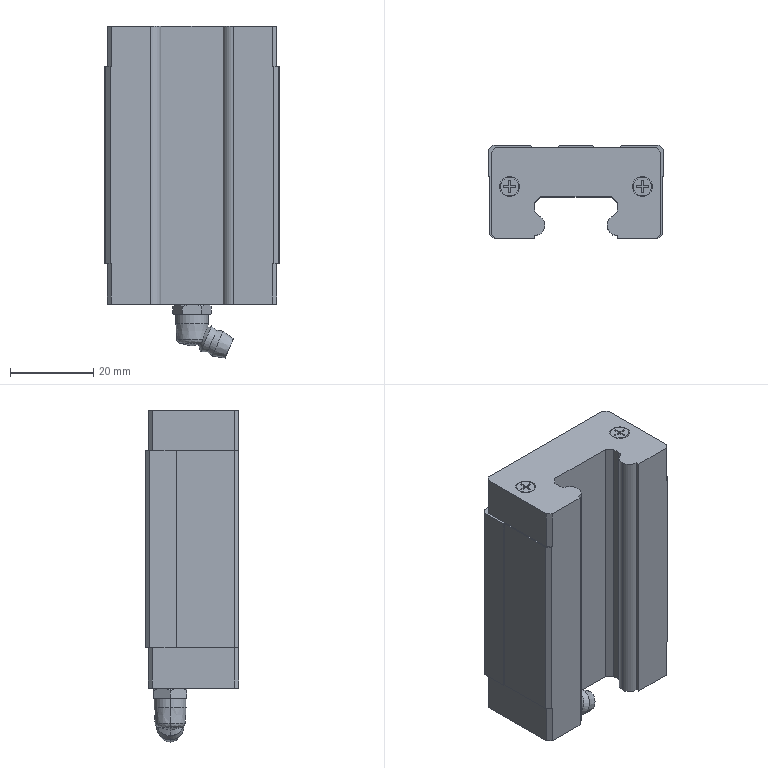Part | STEP file | 0243_Z_SXR28-520_2 | 1 solid | 194 faces | box 42 x 22.5 x 80 mm | volume 49565 mm3 | plane 99 | cylinder 51 | cone 42 | spline 2 | commonest cylinder face diameters 3.08 x20 4.134 x8 4.4 x8 4.8 x8 5 x3 3 x2